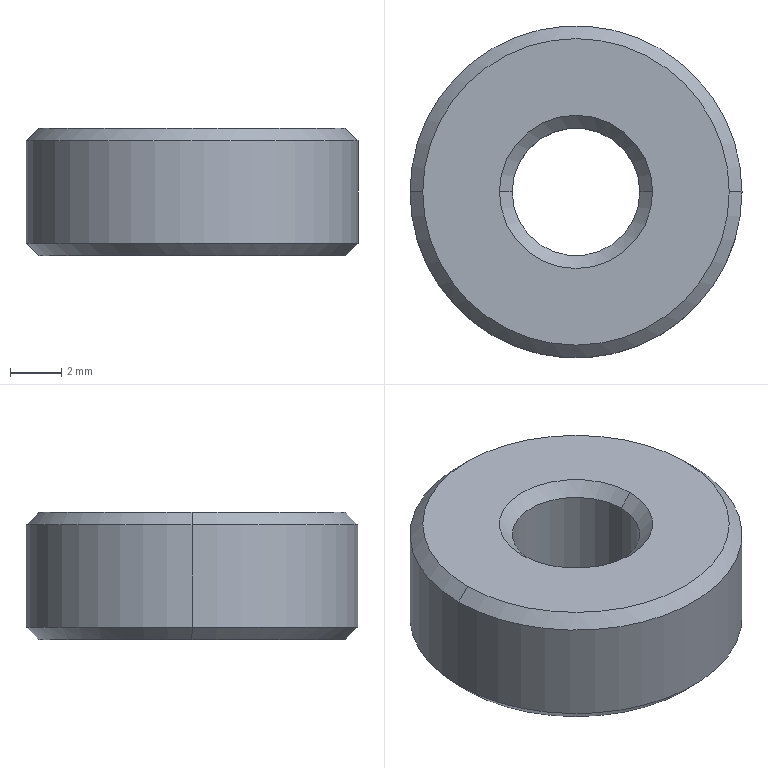Part | STEP file | QA-KGHA5-13 | 1 solid | 14 faces | box 13 x 13 x 5 mm | volume 551.35 mm3 | cone 8 | cylinder 4 | plane 2 | commonest cylinder face diameters 5 x2 13 x2
STEP:
#1=CARTESIAN_POINT('',(0.,0.,0.));
#2=DIRECTION('',(0.,0.,1.));
#3=DIRECTION('',(1.,0.,0.));
#4=AXIS2_PLACEMENT_3D('',#1,#2,#3);
#5=CARTESIAN_POINT('',(6.,0.,5.));
#6=VERTEX_POINT('',#5);
#7=CARTESIAN_POINT('',(-6.,0.,5.));
#8=VERTEX_POINT('',#7);
#9=CARTESIAN_POINT('',(0.,0.,5.));
#10=DIRECTION('',(0.,0.,1.));
#11=DIRECTION('',(1.,0.,0.));
#12=AXIS2_PLACEMENT_3D('',#9,#10,#11);
#13=CIRCLE('',#12,6.);
#14=CARTESIAN_POINT('',(0.,0.,5.));
#15=DIRECTION('',(0.,0.,-1.));
#16=DIRECTION('',(-1.,0.,0.));
#17=AXIS2_PLACEMENT_3D('',#14,#15,#16);
#18=CONICAL_SURFACE('',#17,6.,0.7854);
#19=CARTESIAN_POINT('',(3.142,0.));
#20=DIRECTION('',(-1.,0.));
#21=VECTOR('',#20,1.);
#22=LINE('',#19,#21);
#23=(GEOMETRIC_REPRESENTATION_CONTEXT(2)PARAMETRIC_REPRESENTATION_CONTEXT()REPRESENTATION_CONTEXT('',''));
#24=DEFINITIONAL_REPRESENTATION('',(#22),#23);
#25=PCURVE('',#18,#24);
#26=CARTESIAN_POINT('',(0.,0.,5.));
#27=DIRECTION('',(0.,0.,1.));
#28=DIRECTION('',(1.,0.,0.));
#29=AXIS2_PLACEMENT_3D('',#26,#27,#28);
#30=PLANE('',#29);
#31=CARTESIAN_POINT('',(0.,0.));
#32=DIRECTION('',(1.,0.));
#33=AXIS2_PLACEMENT_2D('',#31,#32);
#34=CIRCLE('',#33,6.);
#35=(GEOMETRIC_REPRESENTATION_CONTEXT(2)PARAMETRIC_REPRESENTATION_CONTEXT()REPRESENTATION_CONTEXT('',''));
#36=DEFINITIONAL_REPRESENTATION('',(#34),#35);
#37=PCURVE('',#30,#36);
#38=SURFACE_CURVE('',#13,(#25,#37),.PCURVE_S1.);
#39=EDGE_CURVE('',#6,#8,#38,.T.);
#40=ORIENTED_EDGE('',*,*,#39,.F.);
#41=CARTESIAN_POINT('',(6.5,0.,4.5));
#42=VERTEX_POINT('',#41);
#43=CARTESIAN_POINT('',(6.,0.,5.));
#44=DIRECTION('',(0.7071,0.,-0.7071));
#45=VECTOR('',#44,1.);
#46=LINE('',#43,#45);
#47=CARTESIAN_POINT('',(3.142,0.));
#48=DIRECTION('',(0.,1.));
#49=VECTOR('',#48,1.);
#50=LINE('',#47,#49);
#51=(GEOMETRIC_REPRESENTATION_CONTEXT(2)PARAMETRIC_REPRESENTATION_CONTEXT()REPRESENTATION_CONTEXT('',''));
#52=DEFINITIONAL_REPRESENTATION('',(#50),#51);
#53=PCURVE('',#18,#52);
#54=CARTESIAN_POINT('',(0.,0.,5.));
#55=DIRECTION('',(0.,0.,-1.));
#56=DIRECTION('',(-1.,0.,0.));
#57=AXIS2_PLACEMENT_3D('',#54,#55,#56);
#58=CONICAL_SURFACE('',#57,6.,0.7854);
#59=CARTESIAN_POINT('',(3.142,0.));
#60=DIRECTION('',(0.,1.));
#61=VECTOR('',#60,1.);
#62=LINE('',#59,#61);
#63=(GEOMETRIC_REPRESENTATION_CONTEXT(2)PARAMETRIC_REPRESENTATION_CONTEXT()REPRESENTATION_CONTEXT('',''));
#64=DEFINITIONAL_REPRESENTATION('',(#62),#63);
#65=PCURVE('',#58,#64);
#66=SURFACE_CURVE('',#46,(#53,#65),.PCURVE_S1.);
#67=EDGE_CURVE('',#6,#42,#66,.T.);
#68=ORIENTED_EDGE('',*,*,#67,.T.);
#69=CARTESIAN_POINT('',(-6.5,0.,4.5));
#70=VERTEX_POINT('',#69);
#71=CARTESIAN_POINT('',(0.,0.,4.5));
#72=DIRECTION('',(0.,0.,-1.));
#73=DIRECTION('',(1.,0.,0.));
#74=AXIS2_PLACEMENT_3D('',#71,#72,#73);
#75=CIRCLE('',#74,6.5);
#76=CARTESIAN_POINT('',(-3.142,0.5));
#77=DIRECTION('',(1.,0.));
#78=VECTOR('',#77,1.);
#79=LINE('',#76,#78);
#80=(GEOMETRIC_REPRESENTATION_CONTEXT(2)PARAMETRIC_REPRESENTATION_CONTEXT()REPRESENTATION_CONTEXT('',''));
#81=DEFINITIONAL_REPRESENTATION('',(#79),#80);
#82=PCURVE('',#18,#81);
#83=CARTESIAN_POINT('',(0.,0.,5.));
#84=DIRECTION('',(0.,0.,-1.));
#85=DIRECTION('',(-1.,0.,0.));
#86=AXIS2_PLACEMENT_3D('',#83,#84,#85);
#87=CYLINDRICAL_SURFACE('',#86,6.5);
#88=CARTESIAN_POINT('',(-3.142,0.5));
#89=DIRECTION('',(1.,0.));
#90=VECTOR('',#89,1.);
#91=LINE('',#88,#90);
#92=(GEOMETRIC_REPRESENTATION_CONTEXT(2)PARAMETRIC_REPRESENTATION_CONTEXT()REPRESENTATION_CONTEXT('',''));
#93=DEFINITIONAL_REPRESENTATION('',(#91),#92);
#94=PCURVE('',#87,#93);
#95=SURFACE_CURVE('',#75,(#82,#94),.PCURVE_S1.);
#96=EDGE_CURVE('',#70,#42,#95,.T.);
#97=ORIENTED_EDGE('',*,*,#96,.F.);
#98=CARTESIAN_POINT('',(-6.,0.,5.));
#99=DIRECTION('',(-0.7071,0.,-0.7071));
#100=VECTOR('',#99,1.);
#101=LINE('',#98,#100);
#102=CARTESIAN_POINT('',(0.,0.));
#103=DIRECTION('',(0.,1.));
#104=VECTOR('',#103,1.);
#105=LINE('',#102,#104);
#106=(GEOMETRIC_REPRESENTATION_CONTEXT(2)PARAMETRIC_REPRESENTATION_CONTEXT()REPRESENTATION_CONTEXT('',''));
#107=DEFINITIONAL_REPRESENTATION('',(#105),#106);
#108=PCURVE('',#18,#107);
#109=CARTESIAN_POINT('',(6.283,0.));
#110=DIRECTION('',(0.,1.));
#111=VECTOR('',#110,1.);
#112=LINE('',#109,#111);
#113=(GEOMETRIC_REPRESENTATION_CONTEXT(2)PARAMETRIC_REPRESENTATION_CONTEXT()REPRESENTATION_CONTEXT('',''));
#114=DEFINITIONAL_REPRESENTATION('',(#112),#113);
#115=PCURVE('',#58,#114);
#116=SURFACE_CURVE('',#101,(#108,#115),.PCURVE_S1.);
#117=EDGE_CURVE('',#8,#70,#116,.T.);
#118=ORIENTED_EDGE('',*,*,#117,.F.);
#119=EDGE_LOOP('',(#40,#68,#97,#118));
#120=FACE_BOUND('',#119,.T.);
#121=ADVANCED_FACE('',(#120),#18,.T.);
#122=CARTESIAN_POINT('',(-6.,0.,0.));
#123=VERTEX_POINT('',#122);
#124=CARTESIAN_POINT('',(6.,0.,0.));
#125=VERTEX_POINT('',#124);
#126=CARTESIAN_POINT('',(0.,0.,0.));
#127=DIRECTION('',(0.,0.,-1.));
#128=DIRECTION('',(1.,0.,0.));
#129=AXIS2_PLACEMENT_3D('',#126,#127,#128);
#130=CIRCLE('',#129,6.);
#131=CARTESIAN_POINT('',(0.,0.,0.5));
#132=DIRECTION('',(0.,0.,1.));
#133=DIRECTION('',(1.,0.,0.));
#134=AXIS2_PLACEMENT_3D('',#131,#132,#133);
#135=CONICAL_SURFACE('',#134,6.5,0.7854);
#136=CARTESIAN_POINT('',(6.283,-0.5));
#137=DIRECTION('',(-1.,0.));
#138=VECTOR('',#137,1.);
#139=LINE('',#136,#138);
#140=(GEOMETRIC_REPRESENTATION_CONTEXT(2)PARAMETRIC_REPRESENTATION_CONTEXT()REPRESENTATION_CONTEXT('',''));
#141=DEFINITIONAL_REPRESENTATION('',(#139),#140);
#142=PCURVE('',#135,#141);
#143=CARTESIAN_POINT('',(0.,0.,0.));
#144=DIRECTION('',(0.,0.,1.));
#145=DIRECTION('',(1.,0.,0.));
#146=AXIS2_PLACEMENT_3D('',#143,#144,#145);
#147=PLANE('',#146);
#148=CARTESIAN_POINT('',(6.,0.));
#149=CARTESIAN_POINT('',(6.,-10.392));
#150=CARTESIAN_POINT('',(-3.,-5.196));
#151=CARTESIAN_POINT('',(-12.,0.));
#152=CARTESIAN_POINT('',(-3.,5.196));
#153=CARTESIAN_POINT('',(6.,10.392));
#154=CARTESIAN_POINT('',(6.,0.));
#155=(BOUNDED_CURVE()B_SPLINE_CURVE(2,(#148,#149,#150,#151,#152,#153,#154),.UNSPECIFIED.,.T.,.F.)B_SPLINE_CURVE_WITH_KNOTS((1,2,2,2,2,1),(-2.094,0.,2.094,4.189,6.283,8.378),.UNSPECIFIED.)CURVE()GEOMETRIC_REPRESENTATION_ITEM()RATIONAL_B_SPLINE_CURVE((1.,0.5,1.,0.5,1.,0.5,1.))REPRESENTATION_ITEM(''));
#156=(GEOMETRIC_REPRESENTATION_CONTEXT(2)PARAMETRIC_REPRESENTATION_CONTEXT()REPRESENTATION_CONTEXT('',''));
#157=DEFINITIONAL_REPRESENTATION('',(#155),#156);
#158=PCURVE('',#147,#157);
#159=SURFACE_CURVE('',#130,(#142,#158),.PCURVE_S1.);
#160=EDGE_CURVE('',#123,#125,#159,.T.);
#161=ORIENTED_EDGE('',*,*,#160,.F.);
#162=CARTESIAN_POINT('',(-6.5,0.,0.5));
#163=VERTEX_POINT('',#162);
#164=CARTESIAN_POINT('',(-6.5,0.,0.5));
#165=DIRECTION('',(-0.7071,0.,0.7071));
#166=VECTOR('',#165,1.);
#167=LINE('',#164,#166);
#168=CARTESIAN_POINT('',(3.142,0.));
#169=DIRECTION('',(0.,1.));
#170=VECTOR('',#169,1.);
#171=LINE('',#168,#170);
#172=(GEOMETRIC_REPRESENTATION_CONTEXT(2)PARAMETRIC_REPRESENTATION_CONTEXT()REPRESENTATION_CONTEXT('',''));
#173=DEFINITIONAL_REPRESENTATION('',(#171),#172);
#174=PCURVE('',#135,#173);
#175=CARTESIAN_POINT('',(0.,0.,0.5));
#176=DIRECTION('',(0.,0.,1.));
#177=DIRECTION('',(1.,0.,0.));
#178=AXIS2_PLACEMENT_3D('',#175,#176,#177);
#179=CONICAL_SURFACE('',#178,6.5,0.7854);
#180=CARTESIAN_POINT('',(3.142,0.));
#181=DIRECTION('',(0.,1.));
#182=VECTOR('',#181,1.);
#183=LINE('',#180,#182);
#184=(GEOMETRIC_REPRESENTATION_CONTEXT(2)PARAMETRIC_REPRESENTATION_CONTEXT()REPRESENTATION_CONTEXT('',''));
#185=DEFINITIONAL_REPRESENTATION('',(#183),#184);
#186=PCURVE('',#179,#185);
#187=SURFACE_CURVE('',#167,(#174,#186),.PCURVE_S1.);
#188=EDGE_CURVE('',#123,#163,#187,.T.);
#189=ORIENTED_EDGE('',*,*,#188,.T.);
#190=CARTESIAN_POINT('',(6.5,0.,0.5));
#191=VERTEX_POINT('',#190);
#192=CARTESIAN_POINT('',(0.,0.,0.5));
#193=DIRECTION('',(0.,0.,1.));
#194=DIRECTION('',(1.,0.,0.));
#195=AXIS2_PLACEMENT_3D('',#192,#193,#194);
#196=CIRCLE('',#195,6.5);
#197=CARTESIAN_POINT('',(0.,0.));
#198=DIRECTION('',(1.,0.));
#199=VECTOR('',#198,1.);
#200=LINE('',#197,#199);
#201=(GEOMETRIC_REPRESENTATION_CONTEXT(2)PARAMETRIC_REPRESENTATION_CONTEXT()REPRESENTATION_CONTEXT('',''));
#202=DEFINITIONAL_REPRESENTATION('',(#200),#201);
#203=PCURVE('',#135,#202);
#204=CARTESIAN_POINT('',(3.142,4.5));
#205=DIRECTION('',(-1.,0.));
#206=VECTOR('',#205,1.);
#207=LINE('',#204,#206);
#208=(GEOMETRIC_REPRESENTATION_CONTEXT(2)PARAMETRIC_REPRESENTATION_CONTEXT()REPRESENTATION_CONTEXT('',''));
#209=DEFINITIONAL_REPRESENTATION('',(#207),#208);
#210=PCURVE('',#87,#209);
#211=SURFACE_CURVE('',#196,(#203,#210),.PCURVE_S1.);
#212=EDGE_CURVE('',#191,#163,#211,.T.);
#213=ORIENTED_EDGE('',*,*,#212,.F.);
#214=CARTESIAN_POINT('',(6.5,0.,0.5));
#215=DIRECTION('',(0.7071,0.,0.7071));
#216=VECTOR('',#215,1.);
#217=LINE('',#214,#216);
#218=CARTESIAN_POINT('',(0.,0.));
#219=DIRECTION('',(0.,1.));
#220=VECTOR('',#219,1.);
#221=LINE('',#218,#220);
#222=(GEOMETRIC_REPRESENTATION_CONTEXT(2)PARAMETRIC_REPRESENTATION_CONTEXT()REPRESENTATION_CONTEXT('',''));
#223=DEFINITIONAL_REPRESENTATION('',(#221),#222);
#224=PCURVE('',#135,#223);
#225=CARTESIAN_POINT('',(6.283,0.));
#226=DIRECTION('',(0.,1.));
#227=VECTOR('',#226,1.);
#228=LINE('',#225,#227);
#229=(GEOMETRIC_REPRESENTATION_CONTEXT(2)PARAMETRIC_REPRESENTATION_CONTEXT()REPRESENTATION_CONTEXT('',''));
#230=DEFINITIONAL_REPRESENTATION('',(#228),#229);
#231=PCURVE('',#179,#230);
#232=SURFACE_CURVE('',#217,(#224,#231),.PCURVE_S1.);
#233=EDGE_CURVE('',#125,#191,#232,.T.);
#234=ORIENTED_EDGE('',*,*,#233,.F.);
#235=EDGE_LOOP('',(#161,#189,#213,#234));
#236=FACE_BOUND('',#235,.T.);
#237=ADVANCED_FACE('',(#236),#135,.T.);
#238=CARTESIAN_POINT('',(2.5,0.,4.5));
#239=VERTEX_POINT('',#238);
#240=CARTESIAN_POINT('',(3.,0.,5.));
#241=VERTEX_POINT('',#240);
#242=CARTESIAN_POINT('',(2.5,0.,4.5));
#243=DIRECTION('',(0.7071,0.,0.7071));
#244=VECTOR('',#243,1.);
#245=LINE('',#242,#244);
#246=CARTESIAN_POINT('',(0.,0.,4.5));
#247=DIRECTION('',(0.,0.,1.));
#248=DIRECTION('',(1.,0.,0.));
#249=AXIS2_PLACEMENT_3D('',#246,#247,#248);
#250=CONICAL_SURFACE('',#249,2.5,0.7854);
#251=CARTESIAN_POINT('',(6.283,0.));
#252=DIRECTION('',(0.,1.));
#253=VECTOR('',#252,1.);
#254=LINE('',#251,#253);
#255=(GEOMETRIC_REPRESENTATION_CONTEXT(2)PARAMETRIC_REPRESENTATION_CONTEXT()REPRESENTATION_CONTEXT('',''));
#256=DEFINITIONAL_REPRESENTATION('',(#254),#255);
#257=PCURVE('',#250,#256);
#258=CARTESIAN_POINT('',(0.,0.,4.5));
#259=DIRECTION('',(0.,0.,1.));
#260=DIRECTION('',(1.,0.,0.));
#261=AXIS2_PLACEMENT_3D('',#258,#259,#260);
#262=CONICAL_SURFACE('',#261,2.5,0.7854);
#263=CARTESIAN_POINT('',(0.,0.));
#264=DIRECTION('',(0.,1.));
#265=VECTOR('',#264,1.);
#266=LINE('',#263,#265);
#267=(GEOMETRIC_REPRESENTATION_CONTEXT(2)PARAMETRIC_REPRESENTATION_CONTEXT()REPRESENTATION_CONTEXT('',''));
#268=DEFINITIONAL_REPRESENTATION('',(#266),#267);
#269=PCURVE('',#262,#268);
#270=SURFACE_CURVE('',#245,(#257,#269),.PCURVE_S1.);
#271=EDGE_CURVE('',#239,#241,#270,.T.);
#272=ORIENTED_EDGE('',*,*,#271,.T.);
#273=CARTESIAN_POINT('',(-3.,0.,5.));
#274=VERTEX_POINT('',#273);
#275=CARTESIAN_POINT('',(0.,0.,5.));
#276=DIRECTION('',(0.,0.,-1.));
#277=DIRECTION('',(1.,0.,0.));
#278=AXIS2_PLACEMENT_3D('',#275,#276,#277);
#279=CIRCLE('',#278,3.);
#280=CARTESIAN_POINT('',(6.283,0.5));
#281=DIRECTION('',(-1.,0.));
#282=VECTOR('',#281,1.);
#283=LINE('',#280,#282);
#284=(GEOMETRIC_REPRESENTATION_CONTEXT(2)PARAMETRIC_REPRESENTATION_CONTEXT()REPRESENTATION_CONTEXT('',''));
#285=DEFINITIONAL_REPRESENTATION('',(#283),#284);
#286=PCURVE('',#250,#285);
#287=CARTESIAN_POINT('',(3.,0.));
#288=CARTESIAN_POINT('',(3.,-5.196));
#289=CARTESIAN_POINT('',(-1.5,-2.598));
#290=CARTESIAN_POINT('',(-6.,0.));
#291=CARTESIAN_POINT('',(-1.5,2.598));
#292=CARTESIAN_POINT('',(3.,5.196));
#293=CARTESIAN_POINT('',(3.,0.));
#294=(BOUNDED_CURVE()B_SPLINE_CURVE(2,(#287,#288,#289,#290,#291,#292,#293),.UNSPECIFIED.,.T.,.F.)B_SPLINE_CURVE_WITH_KNOTS((1,2,2,2,2,1),(-2.094,0.,2.094,4.189,6.283,8.378),.UNSPECIFIED.)CURVE()GEOMETRIC_REPRESENTATION_ITEM()RATIONAL_B_SPLINE_CURVE((1.,0.5,1.,0.5,1.,0.5,1.))REPRESENTATION_ITEM(''));
#295=(GEOMETRIC_REPRESENTATION_CONTEXT(2)PARAMETRIC_REPRESENTATION_CONTEXT()REPRESENTATION_CONTEXT('',''));
#296=DEFINITIONAL_REPRESENTATION('',(#294),#295);
#297=PCURVE('',#30,#296);
#298=SURFACE_CURVE('',#279,(#286,#297),.PCURVE_S1.);
#299=EDGE_CURVE('',#241,#274,#298,.T.);
#300=ORIENTED_EDGE('',*,*,#299,.T.);
#301=CARTESIAN_POINT('',(-2.5,0.,4.5));
#302=VERTEX_POINT('',#301);
#303=CARTESIAN_POINT('',(-2.5,0.,4.5));
#304=DIRECTION('',(-0.7071,0.,0.7071));
#305=VECTOR('',#304,1.);
#306=LINE('',#303,#305);
#307=CARTESIAN_POINT('',(3.142,0.));
#308=DIRECTION('',(0.,1.));
#309=VECTOR('',#308,1.);
#310=LINE('',#307,#309);
#311=(GEOMETRIC_REPRESENTATION_CONTEXT(2)PARAMETRIC_REPRESENTATION_CONTEXT()REPRESENTATION_CONTEXT('',''));
#312=DEFINITIONAL_REPRESENTATION('',(#310),#311);
#313=PCURVE('',#250,#312);
#314=CARTESIAN_POINT('',(3.142,0.));
#315=DIRECTION('',(0.,1.));
#316=VECTOR('',#315,1.);
#317=LINE('',#314,#316);
#318=(GEOMETRIC_REPRESENTATION_CONTEXT(2)PARAMETRIC_REPRESENTATION_CONTEXT()REPRESENTATION_CONTEXT('',''));
#319=DEFINITIONAL_REPRESENTATION('',(#317),#318);
#320=PCURVE('',#262,#319);
#321=SURFACE_CURVE('',#306,(#313,#320),.PCURVE_S1.);
#322=EDGE_CURVE('',#302,#274,#321,.T.);
#323=ORIENTED_EDGE('',*,*,#322,.F.);
#324=CARTESIAN_POINT('',(0.,0.,4.5));
#325=DIRECTION('',(0.,0.,1.));
#326=DIRECTION('',(1.,0.,0.));
#327=AXIS2_PLACEMENT_3D('',#324,#325,#326);
#328=CIRCLE('',#327,2.5);
#329=CARTESIAN_POINT('',(0.,0.));
#330=DIRECTION('',(1.,0.));
#331=VECTOR('',#330,1.);
#332=LINE('',#329,#331);
#333=(GEOMETRIC_REPRESENTATION_CONTEXT(2)PARAMETRIC_REPRESENTATION_CONTEXT()REPRESENTATION_CONTEXT('',''));
#334=DEFINITIONAL_REPRESENTATION('',(#332),#333);
#335=PCURVE('',#250,#334);
#336=CARTESIAN_POINT('',(0.,0.,5.));
#337=DIRECTION('',(0.,0.,-1.));
#338=DIRECTION('',(-1.,0.,0.));
#339=AXIS2_PLACEMENT_3D('',#336,#337,#338);
#340=CYLINDRICAL_SURFACE('',#339,2.5);
#341=CARTESIAN_POINT('',(9.425,0.5));
#342=DIRECTION('',(-1.,0.));
#343=VECTOR('',#342,1.);
#344=LINE('',#341,#343);
#345=(GEOMETRIC_REPRESENTATION_CONTEXT(2)PARAMETRIC_REPRESENTATION_CONTEXT()REPRESENTATION_CONTEXT('',''));
#346=DEFINITIONAL_REPRESENTATION('',(#344),#345);
#347=PCURVE('',#340,#346);
#348=SURFACE_CURVE('',#328,(#335,#347),.PCURVE_S1.);
#349=EDGE_CURVE('',#302,#239,#348,.T.);
#350=ORIENTED_EDGE('',*,*,#349,.T.);
#351=EDGE_LOOP('',(#272,#300,#323,#350));
#352=FACE_BOUND('',#351,.F.);
#353=ADVANCED_FACE('',(#352),#250,.F.);
#354=CARTESIAN_POINT('',(-2.5,0.,0.5));
#355=VERTEX_POINT('',#354);
#356=CARTESIAN_POINT('',(-3.,0.,0.));
#357=VERTEX_POINT('',#356);
#358=CARTESIAN_POINT('',(-3.,0.,0.));
#359=DIRECTION('',(-0.7071,0.,-0.7071));
#360=VECTOR('',#359,1.);
#361=LINE('',#358,#360);
#362=CARTESIAN_POINT('',(0.,0.,0.));
#363=DIRECTION('',(0.,0.,-1.));
#364=DIRECTION('',(-1.,0.,0.));
#365=AXIS2_PLACEMENT_3D('',#362,#363,#364);
#366=CONICAL_SURFACE('',#365,3.,0.7854);
#367=CARTESIAN_POINT('',(6.283,0.));
#368=DIRECTION('',(0.,1.));
#369=VECTOR('',#368,1.);
#370=LINE('',#367,#369);
#371=(GEOMETRIC_REPRESENTATION_CONTEXT(2)PARAMETRIC_REPRESENTATION_CONTEXT()REPRESENTATION_CONTEXT('',''));
#372=DEFINITIONAL_REPRESENTATION('',(#370),#371);
#373=PCURVE('',#366,#372);
#374=CARTESIAN_POINT('',(0.,0.,0.));
#375=DIRECTION('',(0.,0.,-1.));
#376=DIRECTION('',(-1.,0.,0.));
#377=AXIS2_PLACEMENT_3D('',#374,#375,#376);
#378=CONICAL_SURFACE('',#377,3.,0.7854);
#379=CARTESIAN_POINT('',(0.,0.));
#380=DIRECTION('',(0.,1.));
#381=VECTOR('',#380,1.);
#382=LINE('',#379,#381);
#383=(GEOMETRIC_REPRESENTATION_CONTEXT(2)PARAMETRIC_REPRESENTATION_CONTEXT()REPRESENTATION_CONTEXT('',''));
#384=DEFINITIONAL_REPRESENTATION('',(#382),#383);
#385=PCURVE('',#378,#384);
#386=SURFACE_CURVE('',#361,(#373,#385),.PCURVE_S1.);
#387=EDGE_CURVE('',#355,#357,#386,.T.);
#388=ORIENTED_EDGE('',*,*,#387,.T.);
#389=CARTESIAN_POINT('',(3.,0.,0.));
#390=VERTEX_POINT('',#389);
#391=CARTESIAN_POINT('',(0.,0.,0.));
#392=DIRECTION('',(0.,0.,1.));
#393=DIRECTION('',(1.,0.,0.));
#394=AXIS2_PLACEMENT_3D('',#391,#392,#393);
#395=CIRCLE('',#394,3.);
#396=CARTESIAN_POINT('',(9.425,0.));
#397=DIRECTION('',(-1.,0.));
#398=VECTOR('',#397,1.);
#399=LINE('',#396,#398);
#400=(GEOMETRIC_REPRESENTATION_CONTEXT(2)PARAMETRIC_REPRESENTATION_CONTEXT()REPRESENTATION_CONTEXT('',''));
#401=DEFINITIONAL_REPRESENTATION('',(#399),#400);
#402=PCURVE('',#366,#401);
#403=CARTESIAN_POINT('',(0.,0.));
#404=DIRECTION('',(1.,0.));
#405=AXIS2_PLACEMENT_2D('',#403,#404);
#406=CIRCLE('',#405,3.);
#407=(GEOMETRIC_REPRESENTATION_CONTEXT(2)PARAMETRIC_REPRESENTATION_CONTEXT()REPRESENTATION_CONTEXT('',''));
#408=DEFINITIONAL_REPRESENTATION('',(#406),#407);
#409=PCURVE('',#147,#408);
#410=SURFACE_CURVE('',#395,(#402,#409),.PCURVE_S1.);
#411=EDGE_CURVE('',#357,#390,#410,.T.);
#412=ORIENTED_EDGE('',*,*,#411,.T.);
#413=CARTESIAN_POINT('',(2.5,0.,0.5));
#414=VERTEX_POINT('',#413);
#415=CARTESIAN_POINT('',(3.,0.,0.));
#416=DIRECTION('',(0.7071,0.,-0.7071));
#417=VECTOR('',#416,1.);
#418=LINE('',#415,#417);
#419=CARTESIAN_POINT('',(3.142,0.));
#420=DIRECTION('',(0.,1.));
#421=VECTOR('',#420,1.);
#422=LINE('',#419,#421);
#423=(GEOMETRIC_REPRESENTATION_CONTEXT(2)PARAMETRIC_REPRESENTATION_CONTEXT()REPRESENTATION_CONTEXT('',''));
#424=DEFINITIONAL_REPRESENTATION('',(#422),#423);
#425=PCURVE('',#366,#424);
#426=CARTESIAN_POINT('',(3.142,0.));
#427=DIRECTION('',(0.,1.));
#428=VECTOR('',#427,1.);
#429=LINE('',#426,#428);
#430=(GEOMETRIC_REPRESENTATION_CONTEXT(2)PARAMETRIC_REPRESENTATION_CONTEXT()REPRESENTATION_CONTEXT('',''));
#431=DEFINITIONAL_REPRESENTATION('',(#429),#430);
#432=PCURVE('',#378,#431);
#433=SURFACE_CURVE('',#418,(#425,#432),.PCURVE_S1.);
#434=EDGE_CURVE('',#414,#390,#433,.T.);
#435=ORIENTED_EDGE('',*,*,#434,.F.);
#436=CARTESIAN_POINT('',(0.,0.,0.5));
#437=DIRECTION('',(0.,0.,-1.));
#438=DIRECTION('',(1.,0.,0.));
#439=AXIS2_PLACEMENT_3D('',#436,#437,#438);
#440=CIRCLE('',#439,2.5);
#441=CARTESIAN_POINT('',(3.142,-0.5));
#442=DIRECTION('',(1.,0.));
#443=VECTOR('',#442,1.);
#444=LINE('',#441,#443);
#445=(GEOMETRIC_REPRESENTATION_CONTEXT(2)PARAMETRIC_REPRESENTATION_CONTEXT()REPRESENTATION_CONTEXT('',''));
#446=DEFINITIONAL_REPRESENTATION('',(#444),#445);
#447=PCURVE('',#366,#446);
#448=CARTESIAN_POINT('',(3.142,4.5));
#449=DIRECTION('',(1.,0.));
#450=VECTOR('',#449,1.);
#451=LINE('',#448,#450);
#452=(GEOMETRIC_REPRESENTATION_CONTEXT(2)PARAMETRIC_REPRESENTATION_CONTEXT()REPRESENTATION_CONTEXT('',''));
#453=DEFINITIONAL_REPRESENTATION('',(#451),#452);
#454=PCURVE('',#340,#453);
#455=SURFACE_CURVE('',#440,(#447,#454),.PCURVE_S1.);
#456=EDGE_CURVE('',#414,#355,#455,.T.);
#457=ORIENTED_EDGE('',*,*,#456,.T.);
#458=EDGE_LOOP('',(#388,#412,#435,#457));
#459=FACE_BOUND('',#458,.F.);
#460=ADVANCED_FACE('',(#459),#366,.F.);
#461=CARTESIAN_POINT('',(-2.5,0.,5.));
#462=DIRECTION('',(0.,0.,-1.));
#463=VECTOR('',#462,1.);
#464=LINE('',#461,#463);
#465=CARTESIAN_POINT('',(6.283,0.));
#466=DIRECTION('',(0.,1.));
#467=VECTOR('',#466,1.);
#468=LINE('',#465,#467);
#469=(GEOMETRIC_REPRESENTATION_CONTEXT(2)PARAMETRIC_REPRESENTATION_CONTEXT()REPRESENTATION_CONTEXT('',''));
#470=DEFINITIONAL_REPRESENTATION('',(#468),#469);
#471=PCURVE('',#340,#470);
#472=CARTESIAN_POINT('',(0.,0.,5.));
#473=DIRECTION('',(0.,0.,-1.));
#474=DIRECTION('',(-1.,0.,0.));
#475=AXIS2_PLACEMENT_3D('',#472,#473,#474);
#476=CYLINDRICAL_SURFACE('',#475,2.5);
#477=CARTESIAN_POINT('',(0.,0.));
#478=DIRECTION('',(0.,1.));
#479=VECTOR('',#478,1.);
#480=LINE('',#477,#479);
#481=(GEOMETRIC_REPRESENTATION_CONTEXT(2)PARAMETRIC_REPRESENTATION_CONTEXT()REPRESENTATION_CONTEXT('',''));
#482=DEFINITIONAL_REPRESENTATION('',(#480),#481);
#483=PCURVE('',#476,#482);
#484=SURFACE_CURVE('',#464,(#471,#483),.PCURVE_S1.);
#485=EDGE_CURVE('',#302,#355,#484,.T.);
#486=ORIENTED_EDGE('',*,*,#485,.T.);
#487=ORIENTED_EDGE('',*,*,#456,.F.);
#488=CARTESIAN_POINT('',(2.5,0.,5.));
#489=DIRECTION('',(0.,0.,-1.));
#490=VECTOR('',#489,1.);
#491=LINE('',#488,#490);
#492=CARTESIAN_POINT('',(3.142,0.));
#493=DIRECTION('',(0.,1.));
#494=VECTOR('',#493,1.);
#495=LINE('',#492,#494);
#496=(GEOMETRIC_REPRESENTATION_CONTEXT(2)PARAMETRIC_REPRESENTATION_CONTEXT()REPRESENTATION_CONTEXT('',''));
#497=DEFINITIONAL_REPRESENTATION('',(#495),#496);
#498=PCURVE('',#340,#497);
#499=CARTESIAN_POINT('',(3.142,0.));
#500=DIRECTION('',(0.,1.));
#501=VECTOR('',#500,1.);
#502=LINE('',#499,#501);
#503=(GEOMETRIC_REPRESENTATION_CONTEXT(2)PARAMETRIC_REPRESENTATION_CONTEXT()REPRESENTATION_CONTEXT('',''));
#504=DEFINITIONAL_REPRESENTATION('',(#502),#503);
#505=PCURVE('',#476,#504);
#506=SURFACE_CURVE('',#491,(#498,#505),.PCURVE_S1.);
#507=EDGE_CURVE('',#239,#414,#506,.T.);
#508=ORIENTED_EDGE('',*,*,#507,.F.);
#509=ORIENTED_EDGE('',*,*,#349,.F.);
#510=EDGE_LOOP('',(#486,#487,#508,#509));
#511=FACE_BOUND('',#510,.F.);
#512=ADVANCED_FACE('',(#511),#340,.F.);
#513=ORIENTED_EDGE('',*,*,#96,.T.);
#514=CARTESIAN_POINT('',(6.5,0.,5.));
#515=DIRECTION('',(0.,0.,-1.));
#516=VECTOR('',#515,1.);
#517=LINE('',#514,#516);
#518=CARTESIAN_POINT('',(3.142,0.));
#519=DIRECTION('',(0.,1.));
#520=VECTOR('',#519,1.);
#521=LINE('',#518,#520);
#522=(GEOMETRIC_REPRESENTATION_CONTEXT(2)PARAMETRIC_REPRESENTATION_CONTEXT()REPRESENTATION_CONTEXT('',''));
#523=DEFINITIONAL_REPRESENTATION('',(#521),#522);
#524=PCURVE('',#87,#523);
#525=CARTESIAN_POINT('',(0.,0.,5.));
#526=DIRECTION('',(0.,0.,-1.));
#527=DIRECTION('',(-1.,0.,0.));
#528=AXIS2_PLACEMENT_3D('',#525,#526,#527);
#529=CYLINDRICAL_SURFACE('',#528,6.5);
#530=CARTESIAN_POINT('',(3.142,0.));
#531=DIRECTION('',(0.,1.));
#532=VECTOR('',#531,1.);
#533=LINE('',#530,#532);
#534=(GEOMETRIC_REPRESENTATION_CONTEXT(2)PARAMETRIC_REPRESENTATION_CONTEXT()REPRESENTATION_CONTEXT('',''));
#535=DEFINITIONAL_REPRESENTATION('',(#533),#534);
#536=PCURVE('',#529,#535);
#537=SURFACE_CURVE('',#517,(#524,#536),.PCURVE_S1.);
#538=EDGE_CURVE('',#42,#191,#537,.T.);
#539=ORIENTED_EDGE('',*,*,#538,.T.);
#540=ORIENTED_EDGE('',*,*,#212,.T.);
#541=CARTESIAN_POINT('',(-6.5,0.,5.));
#542=DIRECTION('',(0.,0.,-1.));
#543=VECTOR('',#542,1.);
#544=LINE('',#541,#543);
#545=CARTESIAN_POINT('',(0.,0.));
#546=DIRECTION('',(0.,1.));
#547=VECTOR('',#546,1.);
#548=LINE('',#545,#547);
#549=(GEOMETRIC_REPRESENTATION_CONTEXT(2)PARAMETRIC_REPRESENTATION_CONTEXT()REPRESENTATION_CONTEXT('',''));
#550=DEFINITIONAL_REPRESENTATION('',(#548),#549);
#551=PCURVE('',#87,#550);
#552=CARTESIAN_POINT('',(6.283,0.));
#553=DIRECTION('',(0.,1.));
#554=VECTOR('',#553,1.);
#555=LINE('',#552,#554);
#556=(GEOMETRIC_REPRESENTATION_CONTEXT(2)PARAMETRIC_REPRESENTATION_CONTEXT()REPRESENTATION_CONTEXT('',''));
#557=DEFINITIONAL_REPRESENTATION('',(#555),#556);
#558=PCURVE('',#529,#557);
#559=SURFACE_CURVE('',#544,(#551,#558),.PCURVE_S1.);
#560=EDGE_CURVE('',#70,#163,#559,.T.);
#561=ORIENTED_EDGE('',*,*,#560,.F.);
#562=EDGE_LOOP('',(#513,#539,#540,#561));
#563=FACE_BOUND('',#562,.T.);
#564=ADVANCED_FACE('',(#563),#87,.T.);
#565=ORIENTED_EDGE('',*,*,#299,.T.);
#566=CARTESIAN_POINT('',(0.,0.,5.));
#567=DIRECTION('',(0.,0.,-1.));
#568=DIRECTION('',(1.,0.,0.));
#569=AXIS2_PLACEMENT_3D('',#566,#567,#568);
#570=CIRCLE('',#569,3.);
#571=CARTESIAN_POINT('',(3.,0.));
#572=CARTESIAN_POINT('',(3.,-5.196));
#573=CARTESIAN_POINT('',(-1.5,-2.598));
#574=CARTESIAN_POINT('',(-6.,0.));
#575=CARTESIAN_POINT('',(-1.5,2.598));
#576=CARTESIAN_POINT('',(3.,5.196));
#577=CARTESIAN_POINT('',(3.,0.));
#578=(BOUNDED_CURVE()B_SPLINE_CURVE(2,(#571,#572,#573,#574,#575,#576,#577),.UNSPECIFIED.,.T.,.F.)B_SPLINE_CURVE_WITH_KNOTS((1,2,2,2,2,1),(-2.094,0.,2.094,4.189,6.283,8.378),.UNSPECIFIED.)CURVE()GEOMETRIC_REPRESENTATION_ITEM()RATIONAL_B_SPLINE_CURVE((1.,0.5,1.,0.5,1.,0.5,1.))REPRESENTATION_ITEM(''));
#579=(GEOMETRIC_REPRESENTATION_CONTEXT(2)PARAMETRIC_REPRESENTATION_CONTEXT()REPRESENTATION_CONTEXT('',''));
#580=DEFINITIONAL_REPRESENTATION('',(#578),#579);
#581=PCURVE('',#30,#580);
#582=CARTESIAN_POINT('',(6.283,0.5));
#583=DIRECTION('',(-1.,0.));
#584=VECTOR('',#583,1.);
#585=LINE('',#582,#584);
#586=(GEOMETRIC_REPRESENTATION_CONTEXT(2)PARAMETRIC_REPRESENTATION_CONTEXT()REPRESENTATION_CONTEXT('',''));
#587=DEFINITIONAL_REPRESENTATION('',(#585),#586);
#588=PCURVE('',#262,#587);
#589=SURFACE_CURVE('',#570,(#581,#588),.PCURVE_S1.);
#590=EDGE_CURVE('',#274,#241,#589,.T.);
#591=ORIENTED_EDGE('',*,*,#590,.T.);
#592=EDGE_LOOP('',(#565,#591));
#593=FACE_BOUND('',#592,.T.);
#594=CARTESIAN_POINT('',(0.,0.,5.));
#595=DIRECTION('',(0.,0.,1.));
#596=DIRECTION('',(1.,0.,0.));
#597=AXIS2_PLACEMENT_3D('',#594,#595,#596);
#598=CIRCLE('',#597,6.);
#599=CARTESIAN_POINT('',(0.,0.));
#600=DIRECTION('',(1.,0.));
#601=AXIS2_PLACEMENT_2D('',#599,#600);
#602=CIRCLE('',#601,6.);
#603=(GEOMETRIC_REPRESENTATION_CONTEXT(2)PARAMETRIC_REPRESENTATION_CONTEXT()REPRESENTATION_CONTEXT('',''));
#604=DEFINITIONAL_REPRESENTATION('',(#602),#603);
#605=PCURVE('',#30,#604);
#606=CARTESIAN_POINT('',(9.425,0.));
#607=DIRECTION('',(-1.,0.));
#608=VECTOR('',#607,1.);
#609=LINE('',#606,#608);
#610=(GEOMETRIC_REPRESENTATION_CONTEXT(2)PARAMETRIC_REPRESENTATION_CONTEXT()REPRESENTATION_CONTEXT('',''));
#611=DEFINITIONAL_REPRESENTATION('',(#609),#610);
#612=PCURVE('',#58,#611);
#613=SURFACE_CURVE('',#598,(#605,#612),.PCURVE_S1.);
#614=EDGE_CURVE('',#8,#6,#613,.T.);
#615=ORIENTED_EDGE('',*,*,#614,.T.);
#616=ORIENTED_EDGE('',*,*,#39,.T.);
#617=EDGE_LOOP('',(#615,#616));
#618=FACE_BOUND('',#617,.T.);
#619=ADVANCED_FACE('',(#593,#618),#30,.T.);
#620=ORIENTED_EDGE('',*,*,#411,.T.);
#621=CARTESIAN_POINT('',(0.,0.,0.));
#622=DIRECTION('',(0.,0.,1.));
#623=DIRECTION('',(1.,0.,0.));
#624=AXIS2_PLACEMENT_3D('',#621,#622,#623);
#625=CIRCLE('',#624,3.);
#626=CARTESIAN_POINT('',(0.,0.));
#627=DIRECTION('',(1.,0.));
#628=AXIS2_PLACEMENT_2D('',#626,#627);
#629=CIRCLE('',#628,3.);
#630=(GEOMETRIC_REPRESENTATION_CONTEXT(2)PARAMETRIC_REPRESENTATION_CONTEXT()REPRESENTATION_CONTEXT('',''));
#631=DEFINITIONAL_REPRESENTATION('',(#629),#630);
#632=PCURVE('',#147,#631);
#633=CARTESIAN_POINT('',(3.142,0.));
#634=DIRECTION('',(-1.,0.));
#635=VECTOR('',#634,1.);
#636=LINE('',#633,#635);
#637=(GEOMETRIC_REPRESENTATION_CONTEXT(2)PARAMETRIC_REPRESENTATION_CONTEXT()REPRESENTATION_CONTEXT('',''));
#638=DEFINITIONAL_REPRESENTATION('',(#636),#637);
#639=PCURVE('',#378,#638);
#640=SURFACE_CURVE('',#625,(#632,#639),.PCURVE_S1.);
#641=EDGE_CURVE('',#390,#357,#640,.T.);
#642=ORIENTED_EDGE('',*,*,#641,.T.);
#643=EDGE_LOOP('',(#620,#642));
#644=FACE_BOUND('',#643,.T.);
#645=CARTESIAN_POINT('',(0.,0.,0.));
#646=DIRECTION('',(0.,0.,-1.));
#647=DIRECTION('',(1.,0.,0.));
#648=AXIS2_PLACEMENT_3D('',#645,#646,#647);
#649=CIRCLE('',#648,6.);
#650=CARTESIAN_POINT('',(6.,0.));
#651=CARTESIAN_POINT('',(6.,-10.392));
#652=CARTESIAN_POINT('',(-3.,-5.196));
#653=CARTESIAN_POINT('',(-12.,0.));
#654=CARTESIAN_POINT('',(-3.,5.196));
#655=CARTESIAN_POINT('',(6.,10.392));
#656=CARTESIAN_POINT('',(6.,0.));
#657=(BOUNDED_CURVE()B_SPLINE_CURVE(2,(#650,#651,#652,#653,#654,#655,#656),.UNSPECIFIED.,.T.,.F.)B_SPLINE_CURVE_WITH_KNOTS((1,2,2,2,2,1),(-2.094,0.,2.094,4.189,6.283,8.378),.UNSPECIFIED.)CURVE()GEOMETRIC_REPRESENTATION_ITEM()RATIONAL_B_SPLINE_CURVE((1.,0.5,1.,0.5,1.,0.5,1.))REPRESENTATION_ITEM(''));
#658=(GEOMETRIC_REPRESENTATION_CONTEXT(2)PARAMETRIC_REPRESENTATION_CONTEXT()REPRESENTATION_CONTEXT('',''));
#659=DEFINITIONAL_REPRESENTATION('',(#657),#658);
#660=PCURVE('',#147,#659);
#661=CARTESIAN_POINT('',(6.283,-0.5));
#662=DIRECTION('',(-1.,0.));
#663=VECTOR('',#662,1.);
#664=LINE('',#661,#663);
#665=(GEOMETRIC_REPRESENTATION_CONTEXT(2)PARAMETRIC_REPRESENTATION_CONTEXT()REPRESENTATION_CONTEXT('',''));
#666=DEFINITIONAL_REPRESENTATION('',(#664),#665);
#667=PCURVE('',#179,#666);
#668=SURFACE_CURVE('',#649,(#660,#667),.PCURVE_S1.);
#669=EDGE_CURVE('',#125,#123,#668,.T.);
#670=ORIENTED_EDGE('',*,*,#669,.T.);
#671=ORIENTED_EDGE('',*,*,#160,.T.);
#672=EDGE_LOOP('',(#670,#671));
#673=FACE_BOUND('',#672,.T.);
#674=ADVANCED_FACE('',(#644,#673),#147,.F.);
#675=ORIENTED_EDGE('',*,*,#538,.F.);
#676=CARTESIAN_POINT('',(0.,0.,4.5));
#677=DIRECTION('',(0.,0.,-1.));
#678=DIRECTION('',(1.,0.,0.));
#679=AXIS2_PLACEMENT_3D('',#676,#677,#678);
#680=CIRCLE('',#679,6.5);
#681=CARTESIAN_POINT('',(3.142,0.5));
#682=DIRECTION('',(1.,0.));
#683=VECTOR('',#682,1.);
#684=LINE('',#681,#683);
#685=(GEOMETRIC_REPRESENTATION_CONTEXT(2)PARAMETRIC_REPRESENTATION_CONTEXT()REPRESENTATION_CONTEXT('',''));
#686=DEFINITIONAL_REPRESENTATION('',(#684),#685);
#687=PCURVE('',#529,#686);
#688=CARTESIAN_POINT('',(3.142,0.5));
#689=DIRECTION('',(1.,0.));
#690=VECTOR('',#689,1.);
#691=LINE('',#688,#690);
#692=(GEOMETRIC_REPRESENTATION_CONTEXT(2)PARAMETRIC_REPRESENTATION_CONTEXT()REPRESENTATION_CONTEXT('',''));
#693=DEFINITIONAL_REPRESENTATION('',(#691),#692);
#694=PCURVE('',#58,#693);
#695=SURFACE_CURVE('',#680,(#687,#694),.PCURVE_S1.);
#696=EDGE_CURVE('',#42,#70,#695,.T.);
#697=ORIENTED_EDGE('',*,*,#696,.T.);
#698=ORIENTED_EDGE('',*,*,#560,.T.);
#699=CARTESIAN_POINT('',(0.,0.,0.5));
#700=DIRECTION('',(0.,0.,1.));
#701=DIRECTION('',(1.,0.,0.));
#702=AXIS2_PLACEMENT_3D('',#699,#700,#701);
#703=CIRCLE('',#702,6.5);
#704=CARTESIAN_POINT('',(9.425,4.5));
#705=DIRECTION('',(-1.,0.));
#706=VECTOR('',#705,1.);
#707=LINE('',#704,#706);
#708=(GEOMETRIC_REPRESENTATION_CONTEXT(2)PARAMETRIC_REPRESENTATION_CONTEXT()REPRESENTATION_CONTEXT('',''));
#709=DEFINITIONAL_REPRESENTATION('',(#707),#708);
#710=PCURVE('',#529,#709);
#711=CARTESIAN_POINT('',(0.,0.));
#712=DIRECTION('',(1.,0.));
#713=VECTOR('',#712,1.);
#714=LINE('',#711,#713);
#715=(GEOMETRIC_REPRESENTATION_CONTEXT(2)PARAMETRIC_REPRESENTATION_CONTEXT()REPRESENTATION_CONTEXT('',''));
#716=DEFINITIONAL_REPRESENTATION('',(#714),#715);
#717=PCURVE('',#179,#716);
#718=SURFACE_CURVE('',#703,(#710,#717),.PCURVE_S1.);
#719=EDGE_CURVE('',#163,#191,#718,.T.);
#720=ORIENTED_EDGE('',*,*,#719,.T.);
#721=EDGE_LOOP('',(#675,#697,#698,#720));
#722=FACE_BOUND('',#721,.T.);
#723=ADVANCED_FACE('',(#722),#529,.T.);
#724=CARTESIAN_POINT('',(0.,0.,0.5));
#725=DIRECTION('',(0.,0.,-1.));
#726=DIRECTION('',(1.,0.,0.));
#727=AXIS2_PLACEMENT_3D('',#724,#725,#726);
#728=CIRCLE('',#727,2.5);
#729=CARTESIAN_POINT('',(-3.142,4.5));
#730=DIRECTION('',(1.,0.));
#731=VECTOR('',#730,1.);
#732=LINE('',#729,#731);
#733=(GEOMETRIC_REPRESENTATION_CONTEXT(2)PARAMETRIC_REPRESENTATION_CONTEXT()REPRESENTATION_CONTEXT('',''));
#734=DEFINITIONAL_REPRESENTATION('',(#732),#733);
#735=PCURVE('',#476,#734);
#736=CARTESIAN_POINT('',(-3.142,-0.5));
#737=DIRECTION('',(1.,0.));
#738=VECTOR('',#737,1.);
#739=LINE('',#736,#738);
#740=(GEOMETRIC_REPRESENTATION_CONTEXT(2)PARAMETRIC_REPRESENTATION_CONTEXT()REPRESENTATION_CONTEXT('',''));
#741=DEFINITIONAL_REPRESENTATION('',(#739),#740);
#742=PCURVE('',#378,#741);
#743=SURFACE_CURVE('',#728,(#735,#742),.PCURVE_S1.);
#744=EDGE_CURVE('',#355,#414,#743,.T.);
#745=ORIENTED_EDGE('',*,*,#744,.F.);
#746=ORIENTED_EDGE('',*,*,#485,.F.);
#747=CARTESIAN_POINT('',(0.,0.,4.5));
#748=DIRECTION('',(0.,0.,1.));
#749=DIRECTION('',(1.,0.,0.));
#750=AXIS2_PLACEMENT_3D('',#747,#748,#749);
#751=CIRCLE('',#750,2.5);
#752=CARTESIAN_POINT('',(3.142,0.5));
#753=DIRECTION('',(-1.,0.));
#754=VECTOR('',#753,1.);
#755=LINE('',#752,#754);
#756=(GEOMETRIC_REPRESENTATION_CONTEXT(2)PARAMETRIC_REPRESENTATION_CONTEXT()REPRESENTATION_CONTEXT('',''));
#757=DEFINITIONAL_REPRESENTATION('',(#755),#756);
#758=PCURVE('',#476,#757);
#759=CARTESIAN_POINT('',(0.,0.));
#760=DIRECTION('',(1.,0.));
#761=VECTOR('',#760,1.);
#762=LINE('',#759,#761);
#763=(GEOMETRIC_REPRESENTATION_CONTEXT(2)PARAMETRIC_REPRESENTATION_CONTEXT()REPRESENTATION_CONTEXT('',''));
#764=DEFINITIONAL_REPRESENTATION('',(#762),#763);
#765=PCURVE('',#262,#764);
#766=SURFACE_CURVE('',#751,(#758,#765),.PCURVE_S1.);
#767=EDGE_CURVE('',#239,#302,#766,.T.);
#768=ORIENTED_EDGE('',*,*,#767,.F.);
#769=ORIENTED_EDGE('',*,*,#507,.T.);
#770=EDGE_LOOP('',(#745,#746,#768,#769));
#771=FACE_BOUND('',#770,.F.);
#772=ADVANCED_FACE('',(#771),#476,.F.);
#773=ORIENTED_EDGE('',*,*,#641,.T.);
#774=ORIENTED_EDGE('',*,*,#387,.F.);
#775=ORIENTED_EDGE('',*,*,#744,.T.);
#776=ORIENTED_EDGE('',*,*,#434,.T.);
#777=EDGE_LOOP('',(#773,#774,#775,#776));
#778=FACE_BOUND('',#777,.F.);
#779=ADVANCED_FACE('',(#778),#378,.F.);
#780=ORIENTED_EDGE('',*,*,#590,.T.);
#781=ORIENTED_EDGE('',*,*,#271,.F.);
#782=ORIENTED_EDGE('',*,*,#767,.T.);
#783=ORIENTED_EDGE('',*,*,#322,.T.);
#784=EDGE_LOOP('',(#780,#781,#782,#783));
#785=FACE_BOUND('',#784,.F.);
#786=ADVANCED_FACE('',(#785),#262,.F.);
#787=ORIENTED_EDGE('',*,*,#188,.F.);
#788=ORIENTED_EDGE('',*,*,#669,.F.);
#789=ORIENTED_EDGE('',*,*,#233,.T.);
#790=ORIENTED_EDGE('',*,*,#719,.F.);
#791=EDGE_LOOP('',(#787,#788,#789,#790));
#792=FACE_BOUND('',#791,.T.);
#793=ADVANCED_FACE('',(#792),#179,.T.);
#794=ORIENTED_EDGE('',*,*,#67,.F.);
#795=ORIENTED_EDGE('',*,*,#614,.F.);
#796=ORIENTED_EDGE('',*,*,#117,.T.);
#797=ORIENTED_EDGE('',*,*,#696,.F.);
#798=EDGE_LOOP('',(#794,#795,#796,#797));
#799=FACE_BOUND('',#798,.T.);
#800=ADVANCED_FACE('',(#799),#58,.T.);
#801=CLOSED_SHELL('',(#121,#237,#353,#460,#512,#564,#619,#674,#723,#772,#779,#786,#793,#800));
#802=MANIFOLD_SOLID_BREP('',#801);
#803=(LENGTH_UNIT()NAMED_UNIT(*)SI_UNIT(.MILLI.,.METRE.));
#804=UNCERTAINTY_MEASURE_WITH_UNIT(LENGTH_MEASURE(0.0000001),#803,'','');
#805=(NAMED_UNIT(*)PLANE_ANGLE_UNIT()SI_UNIT($,.RADIAN.));
#806=(NAMED_UNIT(*)SI_UNIT($,.STERADIAN.)SOLID_ANGLE_UNIT());
#807=(GEOMETRIC_REPRESENTATION_CONTEXT(3)GLOBAL_UNCERTAINTY_ASSIGNED_CONTEXT((#804))GLOBAL_UNIT_ASSIGNED_CONTEXT((#803,#805,#806))REPRESENTATION_CONTEXT('',''));
#808=ADVANCED_BREP_SHAPE_REPRESENTATION('',(#4,#802),#807);